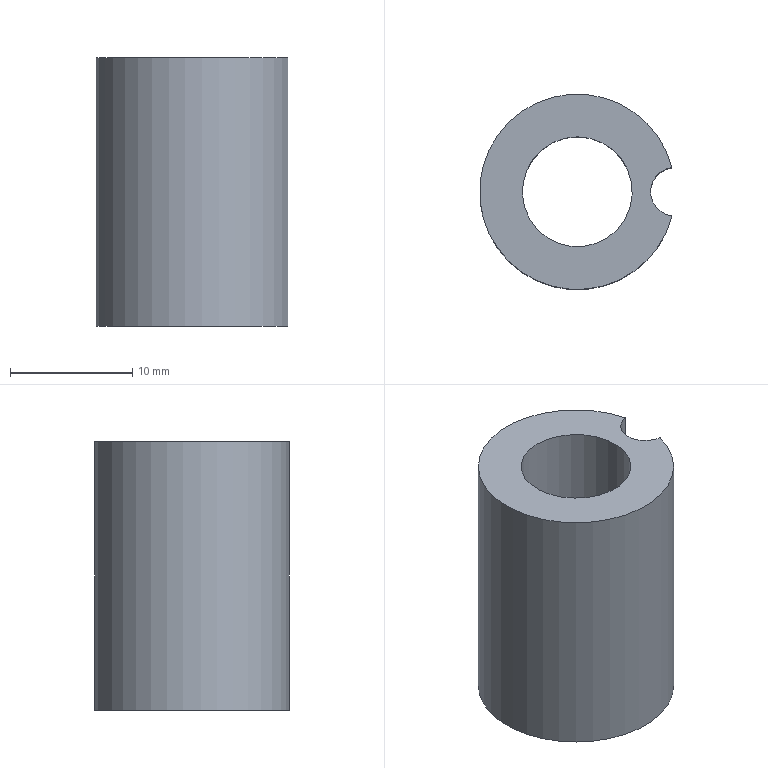Part | NX | features solid 2 | 1 solid | 7 faces | box 15.75 x 16 x 22 mm | volume 2548 mm3 | cylinder 4 | plane 3 | commonest cylinder face diameters 4 x1 9 x1 10.6 x1 16 x1
STEP:
#1=CARTESIAN_POINT('',(820.25,-89.985,29.));
#2=VERTEX_POINT('',#1);
#3=CARTESIAN_POINT('',(820.25,-86.016,29.));
#4=VERTEX_POINT('',#3);
#5=CARTESIAN_POINT('',(820.5,-88.,29.));
#6=DIRECTION('',(0.,0.,-1.));
#7=DIRECTION('',(0.,1.,0.));
#8=AXIS2_PLACEMENT_3D('',#5,#6,#7);
#9=CIRCLE('',#8,2.);
#10=EDGE_CURVE('',#2,#4,#9,.T.);
#11=ORIENTED_EDGE('',*,*,#10,.F.);
#12=CARTESIAN_POINT('',(812.5,-88.,29.));
#13=DIRECTION('',(0.,0.,-1.));
#14=DIRECTION('',(0.,1.,0.));
#15=AXIS2_PLACEMENT_3D('',#12,#13,#14);
#16=CIRCLE('',#15,8.);
#17=EDGE_CURVE('',#2,#4,#16,.T.);
#18=ORIENTED_EDGE('',*,*,#17,.T.);
#19=EDGE_LOOP('',(#11,#18));
#20=FACE_BOUND('',#19,.T.);
#21=CARTESIAN_POINT('',(812.5,-93.3,29.));
#22=VERTEX_POINT('',#21);
#23=CARTESIAN_POINT('',(812.5,-88.,29.));
#24=DIRECTION('',(0.,0.,1.));
#25=DIRECTION('',(0.,-1.,0.));
#26=AXIS2_PLACEMENT_3D('',#23,#24,#25);
#27=CIRCLE('',#26,5.3);
#28=EDGE_CURVE('',#22,#22,#27,.T.);
#29=ORIENTED_EDGE('',*,*,#28,.T.);
#30=EDGE_LOOP('',(#29));
#31=FACE_BOUND('',#30,.T.);
#32=CARTESIAN_POINT('',(812.5,-88.,29.));
#33=DIRECTION('',(0.,0.,-1.));
#34=DIRECTION('',(0.,-1.,0.));
#35=AXIS2_PLACEMENT_3D('',#32,#33,#34);
#36=PLANE('',#35);
#37=ADVANCED_FACE('',(#20,#31),#36,.T.);
#38=CARTESIAN_POINT('',(820.25,-86.016,51.));
#39=VERTEX_POINT('',#38);
#40=CARTESIAN_POINT('',(820.25,-89.985,51.));
#41=VERTEX_POINT('',#40);
#42=CARTESIAN_POINT('',(820.5,-88.,51.));
#43=DIRECTION('',(0.,0.,1.));
#44=DIRECTION('',(0.,-1.,0.));
#45=AXIS2_PLACEMENT_3D('',#42,#43,#44);
#46=CIRCLE('',#45,2.);
#47=EDGE_CURVE('',#39,#41,#46,.T.);
#48=ORIENTED_EDGE('',*,*,#47,.F.);
#49=CARTESIAN_POINT('',(812.5,-88.,51.));
#50=DIRECTION('',(0.,0.,1.));
#51=DIRECTION('',(0.,-1.,0.));
#52=AXIS2_PLACEMENT_3D('',#49,#50,#51);
#53=CIRCLE('',#52,8.);
#54=EDGE_CURVE('',#39,#41,#53,.T.);
#55=ORIENTED_EDGE('',*,*,#54,.T.);
#56=EDGE_LOOP('',(#48,#55));
#57=FACE_BOUND('',#56,.T.);
#58=CARTESIAN_POINT('',(812.5,-83.5,51.));
#59=VERTEX_POINT('',#58);
#60=CARTESIAN_POINT('',(812.5,-88.,51.));
#61=DIRECTION('',(0.,0.,-1.));
#62=DIRECTION('',(0.,1.,0.));
#63=AXIS2_PLACEMENT_3D('',#60,#61,#62);
#64=CIRCLE('',#63,4.5);
#65=EDGE_CURVE('',#59,#59,#64,.T.);
#66=ORIENTED_EDGE('',*,*,#65,.T.);
#67=EDGE_LOOP('',(#66));
#68=FACE_BOUND('',#67,.T.);
#69=CARTESIAN_POINT('',(812.5,-88.,51.));
#70=DIRECTION('',(0.,0.,1.));
#71=DIRECTION('',(0.,1.,0.));
#72=AXIS2_PLACEMENT_3D('',#69,#70,#71);
#73=PLANE('',#72);
#74=ADVANCED_FACE('',(#57,#68),#73,.T.);
#75=CARTESIAN_POINT('',(820.25,-86.016,40.));
#76=DIRECTION('',(0.,0.,-1.));
#77=VECTOR('',#76,1000.);
#78=LINE('',#75,#77);
#79=EDGE_CURVE('',#39,#4,#78,.T.);
#80=ORIENTED_EDGE('',*,*,#79,.T.);
#81=ORIENTED_EDGE('',*,*,#17,.F.);
#82=CARTESIAN_POINT('',(820.25,-89.985,40.));
#83=DIRECTION('',(0.,0.,-1.));
#84=VECTOR('',#83,1000.);
#85=LINE('',#82,#84);
#86=EDGE_CURVE('',#2,#41,#85,.F.);
#87=ORIENTED_EDGE('',*,*,#86,.T.);
#88=ORIENTED_EDGE('',*,*,#54,.F.);
#89=EDGE_LOOP('',(#80,#81,#87,#88));
#90=FACE_BOUND('',#89,.T.);
#91=CARTESIAN_POINT('',(812.5,-88.,51.));
#92=DIRECTION('',(0.,0.,-1.));
#93=DIRECTION('',(0.,-1.,0.));
#94=AXIS2_PLACEMENT_3D('',#91,#92,#93);
#95=CYLINDRICAL_SURFACE('',#94,8.);
#96=ADVANCED_FACE('',(#90),#95,.T.);
#97=CARTESIAN_POINT('',(812.5,-83.5,43.));
#98=VERTEX_POINT('',#97);
#99=CARTESIAN_POINT('',(812.5,-88.,43.));
#100=DIRECTION('',(0.,0.,-1.));
#101=DIRECTION('',(0.,1.,0.));
#102=AXIS2_PLACEMENT_3D('',#99,#100,#101);
#103=CIRCLE('',#102,4.5);
#104=EDGE_CURVE('',#98,#98,#103,.F.);
#105=ORIENTED_EDGE('',*,*,#104,.F.);
#106=EDGE_LOOP('',(#105));
#107=FACE_BOUND('',#106,.T.);
#108=ORIENTED_EDGE('',*,*,#65,.F.);
#109=EDGE_LOOP('',(#108));
#110=FACE_BOUND('',#109,.T.);
#111=CARTESIAN_POINT('',(812.5,-88.,52.));
#112=DIRECTION('',(0.,0.,-1.));
#113=DIRECTION('',(0.,-1.,0.));
#114=AXIS2_PLACEMENT_3D('',#111,#112,#113);
#115=CYLINDRICAL_SURFACE('',#114,4.5);
#116=ADVANCED_FACE('',(#107,#110),#115,.F.);
#117=CARTESIAN_POINT('',(812.5,-93.3,43.));
#118=VERTEX_POINT('',#117);
#119=CARTESIAN_POINT('',(812.5,-88.,43.));
#120=DIRECTION('',(0.,0.,1.));
#121=DIRECTION('',(0.,-1.,0.));
#122=AXIS2_PLACEMENT_3D('',#119,#120,#121);
#123=CIRCLE('',#122,5.3);
#124=EDGE_CURVE('',#118,#118,#123,.T.);
#125=ORIENTED_EDGE('',*,*,#124,.F.);
#126=EDGE_LOOP('',(#125));
#127=FACE_BOUND('',#126,.T.);
#128=ORIENTED_EDGE('',*,*,#104,.T.);
#129=EDGE_LOOP('',(#128));
#130=FACE_BOUND('',#129,.T.);
#131=CARTESIAN_POINT('',(812.5,-88.,43.));
#132=DIRECTION('',(0.,0.,1.));
#133=DIRECTION('',(0.,1.,0.));
#134=AXIS2_PLACEMENT_3D('',#131,#132,#133);
#135=PLANE('',#134);
#136=ADVANCED_FACE('',(#127,#130),#135,.F.);
#137=ORIENTED_EDGE('',*,*,#28,.F.);
#138=EDGE_LOOP('',(#137));
#139=FACE_BOUND('',#138,.T.);
#140=ORIENTED_EDGE('',*,*,#124,.T.);
#141=EDGE_LOOP('',(#140));
#142=FACE_BOUND('',#141,.T.);
#143=CARTESIAN_POINT('',(812.5,-88.,43.));
#144=DIRECTION('',(0.,0.,-1.));
#145=DIRECTION('',(0.,-1.,0.));
#146=AXIS2_PLACEMENT_3D('',#143,#144,#145);
#147=CYLINDRICAL_SURFACE('',#146,5.3);
#148=ADVANCED_FACE('',(#139,#142),#147,.F.);
#149=ORIENTED_EDGE('',*,*,#79,.F.);
#150=ORIENTED_EDGE('',*,*,#47,.T.);
#151=ORIENTED_EDGE('',*,*,#86,.F.);
#152=ORIENTED_EDGE('',*,*,#10,.T.);
#153=EDGE_LOOP('',(#149,#150,#151,#152));
#154=FACE_BOUND('',#153,.T.);
#155=CARTESIAN_POINT('',(820.5,-88.,51.));
#156=DIRECTION('',(0.,0.,-1.));
#157=DIRECTION('',(0.,-1.,0.));
#158=AXIS2_PLACEMENT_3D('',#155,#156,#157);
#159=CYLINDRICAL_SURFACE('',#158,2.);
#160=ADVANCED_FACE('',(#154),#159,.F.);
#161=CLOSED_SHELL('',(#37,#74,#96,#116,#136,#148,#160));
#162=MANIFOLD_SOLID_BREP('',#161);
#163=(LENGTH_UNIT()NAMED_UNIT(*)SI_UNIT(.MILLI.,.METRE.));
#164=UNCERTAINTY_MEASURE_WITH_UNIT(LENGTH_MEASURE(0.00001),#163,'','');
#165=(NAMED_UNIT(*)PLANE_ANGLE_UNIT()SI_UNIT($,.RADIAN.));
#166=(NAMED_UNIT(*)SI_UNIT($,.STERADIAN.)SOLID_ANGLE_UNIT());
#167=(GEOMETRIC_REPRESENTATION_CONTEXT(3)GLOBAL_UNCERTAINTY_ASSIGNED_CONTEXT((#164))GLOBAL_UNIT_ASSIGNED_CONTEXT((#163,#165,#166))REPRESENTATION_CONTEXT('',''));
#168=ADVANCED_BREP_SHAPE_REPRESENTATION('',(#162),#167);